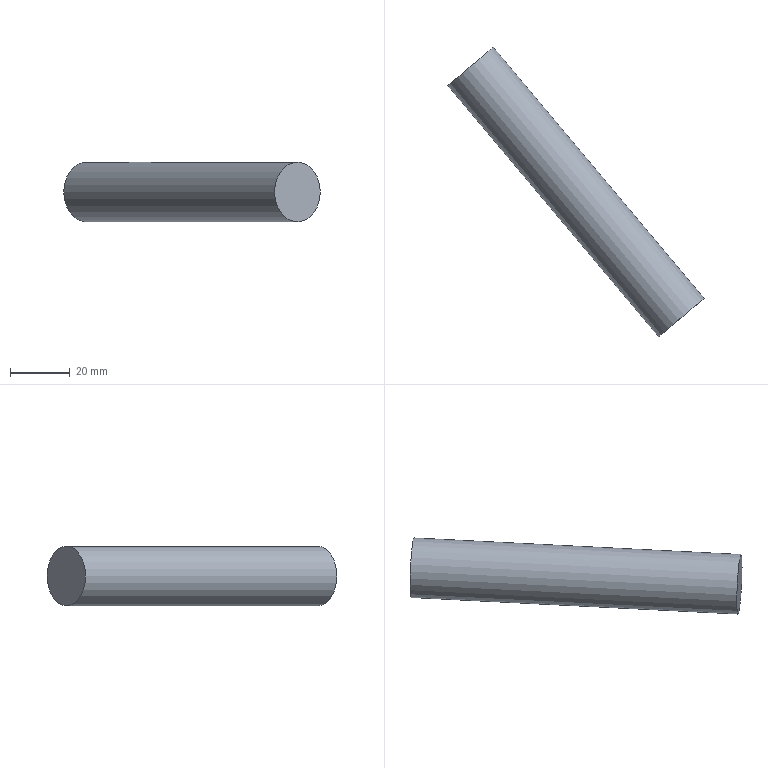Part | NX | features solid 2 | 1 solid | 3 faces | box 86.028 x 97.121 x 20 mm | volume 34558 mm3 | plane 2 | cylinder 1 | commonest cylinder face diameters 20 x1
STEP:
#1=CARTESIAN_POINT('',(793.96,312.901,-50.));
#2=VERTEX_POINT('',#1);
#3=CARTESIAN_POINT('',(801.62,319.329,-50.));
#4=DIRECTION('',(-0.6428,0.766,0.));
#5=DIRECTION('',(-0.766,-0.6428,0.));
#6=AXIS2_PLACEMENT_3D('',#3,#4,#5);
#7=CIRCLE('',#6,10.);
#8=EDGE_CURVE('',#2,#2,#7,.T.);
#9=ORIENTED_EDGE('',*,*,#8,.T.);
#10=EDGE_LOOP('',(#9));
#11=FACE_BOUND('',#10,.T.);
#12=CARTESIAN_POINT('',(723.253,397.166,-50.));
#13=VERTEX_POINT('',#12);
#14=CARTESIAN_POINT('',(730.914,403.594,-50.));
#15=DIRECTION('',(-0.6428,0.766,0.));
#16=DIRECTION('',(-0.766,-0.6428,0.));
#17=AXIS2_PLACEMENT_3D('',#14,#15,#16);
#18=CIRCLE('',#17,10.);
#19=EDGE_CURVE('',#13,#13,#18,.T.);
#20=ORIENTED_EDGE('',*,*,#19,.F.);
#21=EDGE_LOOP('',(#20));
#22=FACE_BOUND('',#21,.T.);
#23=CARTESIAN_POINT('',(801.62,319.329,-50.));
#24=DIRECTION('',(-0.6428,0.766,0.));
#25=DIRECTION('',(0.,0.,-1.));
#26=AXIS2_PLACEMENT_3D('',#23,#24,#25);
#27=CYLINDRICAL_SURFACE('',#26,10.);
#28=ADVANCED_FACE('',(#11,#22),#27,.T.);
#29=ORIENTED_EDGE('',*,*,#8,.F.);
#30=EDGE_LOOP('',(#29));
#31=FACE_BOUND('',#30,.T.);
#32=CARTESIAN_POINT('',(801.62,319.329,-50.));
#33=DIRECTION('',(-0.6428,0.766,0.));
#34=DIRECTION('',(0.,0.,-1.));
#35=AXIS2_PLACEMENT_3D('',#32,#33,#34);
#36=PLANE('',#35);
#37=ADVANCED_FACE('',(#31),#36,.F.);
#38=ORIENTED_EDGE('',*,*,#19,.T.);
#39=EDGE_LOOP('',(#38));
#40=FACE_BOUND('',#39,.T.);
#41=CARTESIAN_POINT('',(730.914,403.594,-50.));
#42=DIRECTION('',(-0.6428,0.766,0.));
#43=DIRECTION('',(0.,0.,-1.));
#44=AXIS2_PLACEMENT_3D('',#41,#42,#43);
#45=PLANE('',#44);
#46=ADVANCED_FACE('',(#40),#45,.T.);
#47=CLOSED_SHELL('',(#28,#37,#46));
#48=MANIFOLD_SOLID_BREP('',#47);
#49=(LENGTH_UNIT()NAMED_UNIT(*)SI_UNIT(.MILLI.,.METRE.));
#50=UNCERTAINTY_MEASURE_WITH_UNIT(LENGTH_MEASURE(0.00001),#49,'','');
#51=(NAMED_UNIT(*)PLANE_ANGLE_UNIT()SI_UNIT($,.RADIAN.));
#52=(NAMED_UNIT(*)SI_UNIT($,.STERADIAN.)SOLID_ANGLE_UNIT());
#53=(GEOMETRIC_REPRESENTATION_CONTEXT(3)GLOBAL_UNCERTAINTY_ASSIGNED_CONTEXT((#50))GLOBAL_UNIT_ASSIGNED_CONTEXT((#49,#51,#52))REPRESENTATION_CONTEXT('',''));
#54=ADVANCED_BREP_SHAPE_REPRESENTATION('',(#48),#53);